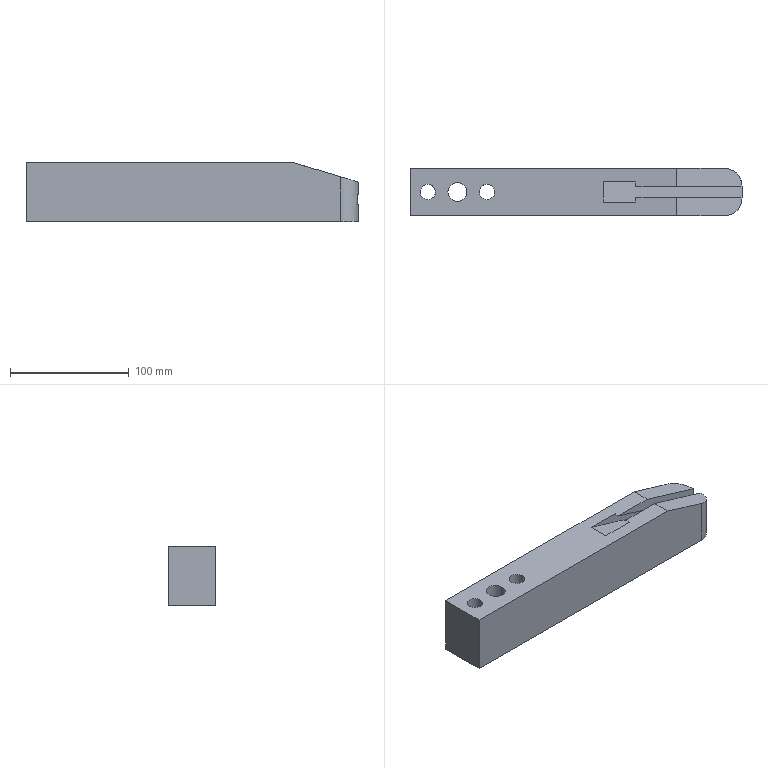Part | STEP file | solid 235 | 1 solid | 26 faces | box 280 x 40 x 50 mm | volume 488862 mm3 | plane 19 | cylinder 7 | commonest cylinder face diameters 13 x2 20 x2 30 x2 16 x1